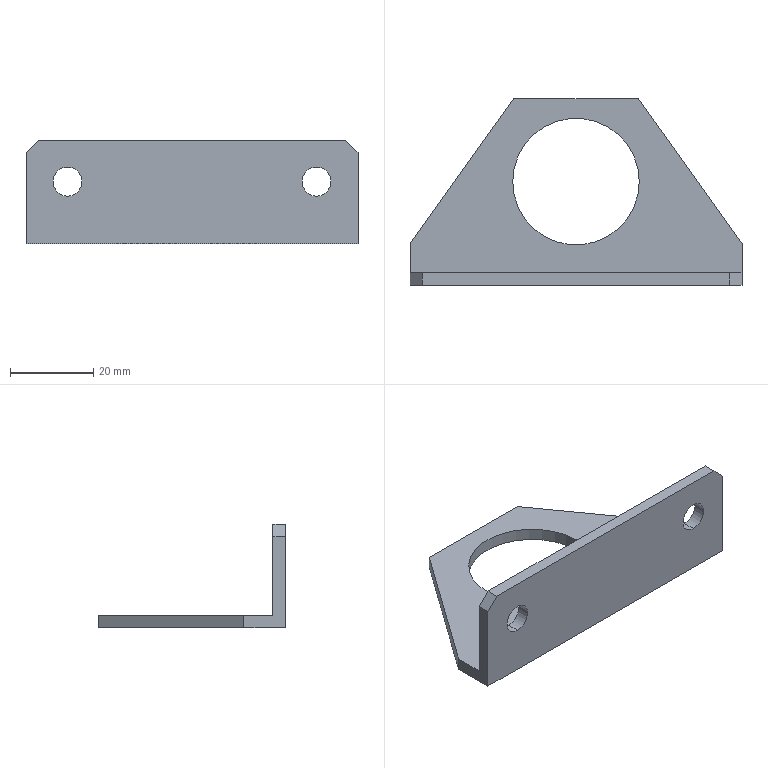Part | SolidWorks | features MBimport 1 | 1 solid | 18 faces | box 80 x 45 x 25 mm | volume 11005 mm3 | plane 12 | cylinder 6 | commonest cylinder face diameters 7 x4 30.5 x2
STEP:
#1=CARTESIAN_POINT('',(30.,3.,18.5));
#2=VERTEX_POINT('',#1);
#3=CARTESIAN_POINT('',(30.,0.,18.5));
#4=VERTEX_POINT('',#3);
#5=CARTESIAN_POINT('',(30.,3.,18.5));
#6=DIRECTION('',(0.,-1.,0.));
#7=VECTOR('',#6,1000.);
#8=LINE('',#5,#7);
#9=EDGE_CURVE('',#2,#4,#8,.T.);
#10=ORIENTED_EDGE('',*,*,#9,.F.);
#11=CARTESIAN_POINT('',(30.,3.,11.5));
#12=VERTEX_POINT('',#11);
#13=CARTESIAN_POINT('',(30.,3.,15.));
#14=DIRECTION('',(0.,-1.,0.));
#15=DIRECTION('',(0.,0.,-1.));
#16=AXIS2_PLACEMENT_3D('',#13,#14,#15);
#17=CIRCLE('',#16,3.5);
#18=EDGE_CURVE('',#12,#2,#17,.T.);
#19=ORIENTED_EDGE('',*,*,#18,.F.);
#20=CARTESIAN_POINT('',(30.,0.,11.5));
#21=VERTEX_POINT('',#20);
#22=CARTESIAN_POINT('',(30.,3.,11.5));
#23=DIRECTION('',(0.,-1.,0.));
#24=VECTOR('',#23,1000.);
#25=LINE('',#22,#24);
#26=EDGE_CURVE('',#12,#21,#25,.T.);
#27=ORIENTED_EDGE('',*,*,#26,.T.);
#28=CARTESIAN_POINT('',(30.,0.,15.));
#29=DIRECTION('',(0.,-1.,0.));
#30=DIRECTION('',(0.,0.,-1.));
#31=AXIS2_PLACEMENT_3D('',#28,#29,#30);
#32=CIRCLE('',#31,3.5);
#33=EDGE_CURVE('',#21,#4,#32,.T.);
#34=ORIENTED_EDGE('',*,*,#33,.T.);
#35=EDGE_LOOP('',(#10,#19,#27,#34));
#36=FACE_OUTER_BOUND('',#35,.T.);
#37=CARTESIAN_POINT('',(30.,3.,15.));
#38=DIRECTION('',(0.,-1.,0.));
#39=DIRECTION('',(0.,0.,-1.));
#40=AXIS2_PLACEMENT_3D('',#37,#38,#39);
#41=CYLINDRICAL_SURFACE('',#40,3.5);
#42=ADVANCED_FACE('',(#36),#41,.F.);
#43=CARTESIAN_POINT('',(-30.,3.,18.5));
#44=VERTEX_POINT('',#43);
#45=CARTESIAN_POINT('',(-30.,0.,18.5));
#46=VERTEX_POINT('',#45);
#47=CARTESIAN_POINT('',(-30.,3.,18.5));
#48=DIRECTION('',(0.,-1.,0.));
#49=VECTOR('',#48,1000.);
#50=LINE('',#47,#49);
#51=EDGE_CURVE('',#44,#46,#50,.T.);
#52=ORIENTED_EDGE('',*,*,#51,.F.);
#53=CARTESIAN_POINT('',(-30.,3.,11.5));
#54=VERTEX_POINT('',#53);
#55=CARTESIAN_POINT('',(-30.,3.,15.));
#56=DIRECTION('',(0.,-1.,0.));
#57=DIRECTION('',(0.,0.,-1.));
#58=AXIS2_PLACEMENT_3D('',#55,#56,#57);
#59=CIRCLE('',#58,3.5);
#60=EDGE_CURVE('',#54,#44,#59,.T.);
#61=ORIENTED_EDGE('',*,*,#60,.F.);
#62=CARTESIAN_POINT('',(-30.,0.,11.5));
#63=VERTEX_POINT('',#62);
#64=CARTESIAN_POINT('',(-30.,3.,11.5));
#65=DIRECTION('',(0.,-1.,0.));
#66=VECTOR('',#65,1000.);
#67=LINE('',#64,#66);
#68=EDGE_CURVE('',#54,#63,#67,.T.);
#69=ORIENTED_EDGE('',*,*,#68,.T.);
#70=CARTESIAN_POINT('',(-30.,0.,15.));
#71=DIRECTION('',(0.,-1.,0.));
#72=DIRECTION('',(0.,0.,-1.));
#73=AXIS2_PLACEMENT_3D('',#70,#71,#72);
#74=CIRCLE('',#73,3.5);
#75=EDGE_CURVE('',#63,#46,#74,.T.);
#76=ORIENTED_EDGE('',*,*,#75,.T.);
#77=EDGE_LOOP('',(#52,#61,#69,#76));
#78=FACE_OUTER_BOUND('',#77,.T.);
#79=CARTESIAN_POINT('',(-30.,3.,15.));
#80=DIRECTION('',(0.,-1.,0.));
#81=DIRECTION('',(0.,0.,-1.));
#82=AXIS2_PLACEMENT_3D('',#79,#80,#81);
#83=CYLINDRICAL_SURFACE('',#82,3.5);
#84=ADVANCED_FACE('',(#78),#83,.F.);
#85=ORIENTED_EDGE('',*,*,#60,.T.);
#86=CARTESIAN_POINT('',(-30.,3.,15.));
#87=DIRECTION('',(0.,-1.,0.));
#88=DIRECTION('',(0.,0.,-1.));
#89=AXIS2_PLACEMENT_3D('',#86,#87,#88);
#90=CIRCLE('',#89,3.5);
#91=EDGE_CURVE('',#44,#54,#90,.T.);
#92=ORIENTED_EDGE('',*,*,#91,.T.);
#93=EDGE_LOOP('',(#85,#92));
#94=FACE_BOUND('',#93,.T.);
#95=ORIENTED_EDGE('',*,*,#18,.T.);
#96=CARTESIAN_POINT('',(30.,3.,15.));
#97=DIRECTION('',(0.,-1.,0.));
#98=DIRECTION('',(0.,0.,-1.));
#99=AXIS2_PLACEMENT_3D('',#96,#97,#98);
#100=CIRCLE('',#99,3.5);
#101=EDGE_CURVE('',#2,#12,#100,.T.);
#102=ORIENTED_EDGE('',*,*,#101,.T.);
#103=EDGE_LOOP('',(#95,#102));
#104=FACE_BOUND('',#103,.T.);
#105=CARTESIAN_POINT('',(-40.,3.,3.));
#106=VERTEX_POINT('',#105);
#107=CARTESIAN_POINT('',(40.,3.,3.));
#108=VERTEX_POINT('',#107);
#109=CARTESIAN_POINT('',(0.,3.,3.));
#110=DIRECTION('',(1.,0.,0.));
#111=VECTOR('',#110,1000.);
#112=LINE('',#109,#111);
#113=EDGE_CURVE('',#106,#108,#112,.T.);
#114=ORIENTED_EDGE('',*,*,#113,.F.);
#115=CARTESIAN_POINT('',(-40.,3.,22.));
#116=VERTEX_POINT('',#115);
#117=CARTESIAN_POINT('',(-40.,3.,0.));
#118=DIRECTION('',(0.,0.,-1.));
#119=VECTOR('',#118,1000.);
#120=LINE('',#117,#119);
#121=EDGE_CURVE('',#116,#106,#120,.T.);
#122=ORIENTED_EDGE('',*,*,#121,.F.);
#123=CARTESIAN_POINT('',(-37.,3.,25.));
#124=VERTEX_POINT('',#123);
#125=CARTESIAN_POINT('',(-40.,3.,22.));
#126=DIRECTION('',(-0.7071,0.,-0.7071));
#127=VECTOR('',#126,1000.);
#128=LINE('',#125,#127);
#129=EDGE_CURVE('',#124,#116,#128,.T.);
#130=ORIENTED_EDGE('',*,*,#129,.F.);
#131=CARTESIAN_POINT('',(37.,3.,25.));
#132=VERTEX_POINT('',#131);
#133=CARTESIAN_POINT('',(-37.,3.,25.));
#134=DIRECTION('',(-1.,0.,0.));
#135=VECTOR('',#134,1000.);
#136=LINE('',#133,#135);
#137=EDGE_CURVE('',#132,#124,#136,.T.);
#138=ORIENTED_EDGE('',*,*,#137,.F.);
#139=CARTESIAN_POINT('',(40.,3.,22.));
#140=VERTEX_POINT('',#139);
#141=CARTESIAN_POINT('',(37.,3.,25.));
#142=DIRECTION('',(-0.7071,0.,0.7071));
#143=VECTOR('',#142,1000.);
#144=LINE('',#141,#143);
#145=EDGE_CURVE('',#140,#132,#144,.T.);
#146=ORIENTED_EDGE('',*,*,#145,.F.);
#147=CARTESIAN_POINT('',(40.,3.,0.));
#148=DIRECTION('',(0.,0.,1.));
#149=VECTOR('',#148,1000.);
#150=LINE('',#147,#149);
#151=EDGE_CURVE('',#108,#140,#150,.T.);
#152=ORIENTED_EDGE('',*,*,#151,.F.);
#153=EDGE_LOOP('',(#114,#122,#130,#138,#146,#152));
#154=FACE_OUTER_BOUND('',#153,.T.);
#155=CARTESIAN_POINT('',(0.,3.,0.));
#156=DIRECTION('',(0.,-1.,0.));
#157=DIRECTION('',(0.,0.,-1.));
#158=AXIS2_PLACEMENT_3D('',#155,#156,#157);
#159=PLANE('',#158);
#160=ADVANCED_FACE('',(#94,#104,#154),#159,.F.);
#161=CARTESIAN_POINT('',(40.,0.,22.));
#162=VERTEX_POINT('',#161);
#163=CARTESIAN_POINT('',(37.,0.,25.));
#164=VERTEX_POINT('',#163);
#165=CARTESIAN_POINT('',(37.,0.,25.));
#166=DIRECTION('',(-0.7071,0.,0.7071));
#167=VECTOR('',#166,1000.);
#168=LINE('',#165,#167);
#169=EDGE_CURVE('',#162,#164,#168,.T.);
#170=ORIENTED_EDGE('',*,*,#169,.F.);
#171=CARTESIAN_POINT('',(40.,3.,22.));
#172=DIRECTION('',(0.,-1.,0.));
#173=VECTOR('',#172,1000.);
#174=LINE('',#171,#173);
#175=EDGE_CURVE('',#140,#162,#174,.T.);
#176=ORIENTED_EDGE('',*,*,#175,.F.);
#177=ORIENTED_EDGE('',*,*,#145,.T.);
#178=CARTESIAN_POINT('',(37.,3.,25.));
#179=DIRECTION('',(0.,-1.,0.));
#180=VECTOR('',#179,1000.);
#181=LINE('',#178,#180);
#182=EDGE_CURVE('',#132,#164,#181,.T.);
#183=ORIENTED_EDGE('',*,*,#182,.T.);
#184=EDGE_LOOP('',(#170,#176,#177,#183));
#185=FACE_OUTER_BOUND('',#184,.T.);
#186=CARTESIAN_POINT('',(37.,3.,25.));
#187=DIRECTION('',(0.7071,0.,0.7071));
#188=DIRECTION('',(0.,-1.,0.));
#189=AXIS2_PLACEMENT_3D('',#186,#187,#188);
#190=PLANE('',#189);
#191=ADVANCED_FACE('',(#185),#190,.T.);
#192=CARTESIAN_POINT('',(-37.,0.,25.));
#193=VERTEX_POINT('',#192);
#194=CARTESIAN_POINT('',(-37.,0.,25.));
#195=DIRECTION('',(-1.,0.,0.));
#196=VECTOR('',#195,1000.);
#197=LINE('',#194,#196);
#198=EDGE_CURVE('',#164,#193,#197,.T.);
#199=ORIENTED_EDGE('',*,*,#198,.F.);
#200=ORIENTED_EDGE('',*,*,#182,.F.);
#201=ORIENTED_EDGE('',*,*,#137,.T.);
#202=CARTESIAN_POINT('',(-37.,3.,25.));
#203=DIRECTION('',(0.,-1.,0.));
#204=VECTOR('',#203,1000.);
#205=LINE('',#202,#204);
#206=EDGE_CURVE('',#124,#193,#205,.T.);
#207=ORIENTED_EDGE('',*,*,#206,.T.);
#208=EDGE_LOOP('',(#199,#200,#201,#207));
#209=FACE_OUTER_BOUND('',#208,.T.);
#210=CARTESIAN_POINT('',(-37.,3.,25.));
#211=DIRECTION('',(0.,0.,1.));
#212=DIRECTION('',(1.,0.,0.));
#213=AXIS2_PLACEMENT_3D('',#210,#211,#212);
#214=PLANE('',#213);
#215=ADVANCED_FACE('',(#209),#214,.T.);
#216=CARTESIAN_POINT('',(-40.,0.,22.));
#217=VERTEX_POINT('',#216);
#218=CARTESIAN_POINT('',(-40.,0.,22.));
#219=DIRECTION('',(-0.7071,0.,-0.7071));
#220=VECTOR('',#219,1000.);
#221=LINE('',#218,#220);
#222=EDGE_CURVE('',#193,#217,#221,.T.);
#223=ORIENTED_EDGE('',*,*,#222,.F.);
#224=ORIENTED_EDGE('',*,*,#206,.F.);
#225=ORIENTED_EDGE('',*,*,#129,.T.);
#226=CARTESIAN_POINT('',(-40.,3.,22.));
#227=DIRECTION('',(0.,-1.,0.));
#228=VECTOR('',#227,1000.);
#229=LINE('',#226,#228);
#230=EDGE_CURVE('',#116,#217,#229,.T.);
#231=ORIENTED_EDGE('',*,*,#230,.T.);
#232=EDGE_LOOP('',(#223,#224,#225,#231));
#233=FACE_OUTER_BOUND('',#232,.T.);
#234=CARTESIAN_POINT('',(-40.,3.,22.));
#235=DIRECTION('',(-0.7071,0.,0.7071));
#236=DIRECTION('',(0.,1.,0.));
#237=AXIS2_PLACEMENT_3D('',#234,#235,#236);
#238=PLANE('',#237);
#239=ADVANCED_FACE('',(#233),#238,.T.);
#240=CARTESIAN_POINT('',(15.25,25.,3.));
#241=VERTEX_POINT('',#240);
#242=CARTESIAN_POINT('',(15.25,25.,0.));
#243=VERTEX_POINT('',#242);
#244=CARTESIAN_POINT('',(15.25,25.,3.));
#245=DIRECTION('',(0.,0.,-1.));
#246=VECTOR('',#245,1000.);
#247=LINE('',#244,#246);
#248=EDGE_CURVE('',#241,#243,#247,.T.);
#249=ORIENTED_EDGE('',*,*,#248,.F.);
#250=CARTESIAN_POINT('',(-15.25,25.,3.));
#251=VERTEX_POINT('',#250);
#252=CARTESIAN_POINT('',(0.,25.,3.));
#253=DIRECTION('',(0.,0.,1.));
#254=DIRECTION('',(1.,0.,0.));
#255=AXIS2_PLACEMENT_3D('',#252,#253,#254);
#256=CIRCLE('',#255,15.25);
#257=EDGE_CURVE('',#241,#251,#256,.T.);
#258=ORIENTED_EDGE('',*,*,#257,.T.);
#259=CARTESIAN_POINT('',(-15.25,25.,0.));
#260=VERTEX_POINT('',#259);
#261=CARTESIAN_POINT('',(-15.25,25.,3.));
#262=DIRECTION('',(0.,0.,-1.));
#263=VECTOR('',#262,1000.);
#264=LINE('',#261,#263);
#265=EDGE_CURVE('',#251,#260,#264,.T.);
#266=ORIENTED_EDGE('',*,*,#265,.T.);
#267=CARTESIAN_POINT('',(0.,25.,0.));
#268=DIRECTION('',(0.,0.,1.));
#269=DIRECTION('',(1.,0.,0.));
#270=AXIS2_PLACEMENT_3D('',#267,#268,#269);
#271=CIRCLE('',#270,15.25);
#272=EDGE_CURVE('',#243,#260,#271,.T.);
#273=ORIENTED_EDGE('',*,*,#272,.F.);
#274=EDGE_LOOP('',(#249,#258,#266,#273));
#275=FACE_OUTER_BOUND('',#274,.T.);
#276=CARTESIAN_POINT('',(0.,25.,3.));
#277=DIRECTION('',(0.,0.,-1.));
#278=DIRECTION('',(-1.,0.,0.));
#279=AXIS2_PLACEMENT_3D('',#276,#277,#278);
#280=CYLINDRICAL_SURFACE('',#279,15.25);
#281=ADVANCED_FACE('',(#275),#280,.F.);
#282=CARTESIAN_POINT('',(-15.,45.,0.));
#283=VERTEX_POINT('',#282);
#284=CARTESIAN_POINT('',(-40.,10.,0.));
#285=VERTEX_POINT('',#284);
#286=CARTESIAN_POINT('',(-15.,45.,0.));
#287=DIRECTION('',(-0.5812,-0.8137,0.));
#288=VECTOR('',#287,1000.);
#289=LINE('',#286,#288);
#290=EDGE_CURVE('',#283,#285,#289,.T.);
#291=ORIENTED_EDGE('',*,*,#290,.T.);
#292=CARTESIAN_POINT('',(-40.,10.,3.));
#293=VERTEX_POINT('',#292);
#294=CARTESIAN_POINT('',(-40.,10.,3.));
#295=DIRECTION('',(0.,0.,-1.));
#296=VECTOR('',#295,1000.);
#297=LINE('',#294,#296);
#298=EDGE_CURVE('',#293,#285,#297,.T.);
#299=ORIENTED_EDGE('',*,*,#298,.F.);
#300=CARTESIAN_POINT('',(-15.,45.,3.));
#301=VERTEX_POINT('',#300);
#302=CARTESIAN_POINT('',(-15.,45.,3.));
#303=DIRECTION('',(-0.5812,-0.8137,0.));
#304=VECTOR('',#303,1000.);
#305=LINE('',#302,#304);
#306=EDGE_CURVE('',#301,#293,#305,.T.);
#307=ORIENTED_EDGE('',*,*,#306,.F.);
#308=CARTESIAN_POINT('',(-15.,45.,3.));
#309=DIRECTION('',(0.,0.,-1.));
#310=VECTOR('',#309,1000.);
#311=LINE('',#308,#310);
#312=EDGE_CURVE('',#301,#283,#311,.T.);
#313=ORIENTED_EDGE('',*,*,#312,.T.);
#314=EDGE_LOOP('',(#291,#299,#307,#313));
#315=FACE_OUTER_BOUND('',#314,.T.);
#316=CARTESIAN_POINT('',(-15.,45.,3.));
#317=DIRECTION('',(0.8137,-0.5812,0.));
#318=DIRECTION('',(0.,0.,-1.));
#319=AXIS2_PLACEMENT_3D('',#316,#317,#318);
#320=PLANE('',#319);
#321=ADVANCED_FACE('',(#315),#320,.F.);
#322=CARTESIAN_POINT('',(15.,45.,0.));
#323=VERTEX_POINT('',#322);
#324=CARTESIAN_POINT('',(15.,45.,0.));
#325=DIRECTION('',(-1.,0.,0.));
#326=VECTOR('',#325,1000.);
#327=LINE('',#324,#326);
#328=EDGE_CURVE('',#323,#283,#327,.T.);
#329=ORIENTED_EDGE('',*,*,#328,.T.);
#330=ORIENTED_EDGE('',*,*,#312,.F.);
#331=CARTESIAN_POINT('',(15.,45.,3.));
#332=VERTEX_POINT('',#331);
#333=CARTESIAN_POINT('',(15.,45.,3.));
#334=DIRECTION('',(-1.,0.,0.));
#335=VECTOR('',#334,1000.);
#336=LINE('',#333,#335);
#337=EDGE_CURVE('',#332,#301,#336,.T.);
#338=ORIENTED_EDGE('',*,*,#337,.F.);
#339=CARTESIAN_POINT('',(15.,45.,3.));
#340=DIRECTION('',(0.,0.,-1.));
#341=VECTOR('',#340,1000.);
#342=LINE('',#339,#341);
#343=EDGE_CURVE('',#332,#323,#342,.T.);
#344=ORIENTED_EDGE('',*,*,#343,.T.);
#345=EDGE_LOOP('',(#329,#330,#338,#344));
#346=FACE_OUTER_BOUND('',#345,.T.);
#347=CARTESIAN_POINT('',(15.,45.,3.));
#348=DIRECTION('',(0.,-1.,0.));
#349=DIRECTION('',(0.,0.,-1.));
#350=AXIS2_PLACEMENT_3D('',#347,#348,#349);
#351=PLANE('',#350);
#352=ADVANCED_FACE('',(#346),#351,.F.);
#353=CARTESIAN_POINT('',(40.,10.,0.));
#354=VERTEX_POINT('',#353);
#355=CARTESIAN_POINT('',(40.,10.,0.));
#356=DIRECTION('',(-0.5812,0.8137,0.));
#357=VECTOR('',#356,1000.);
#358=LINE('',#355,#357);
#359=EDGE_CURVE('',#354,#323,#358,.T.);
#360=ORIENTED_EDGE('',*,*,#359,.T.);
#361=ORIENTED_EDGE('',*,*,#343,.F.);
#362=CARTESIAN_POINT('',(40.,10.,3.));
#363=VERTEX_POINT('',#362);
#364=CARTESIAN_POINT('',(40.,10.,3.));
#365=DIRECTION('',(-0.5812,0.8137,0.));
#366=VECTOR('',#365,1000.);
#367=LINE('',#364,#366);
#368=EDGE_CURVE('',#363,#332,#367,.T.);
#369=ORIENTED_EDGE('',*,*,#368,.F.);
#370=CARTESIAN_POINT('',(40.,10.,3.));
#371=DIRECTION('',(0.,0.,-1.));
#372=VECTOR('',#371,1000.);
#373=LINE('',#370,#372);
#374=EDGE_CURVE('',#363,#354,#373,.T.);
#375=ORIENTED_EDGE('',*,*,#374,.T.);
#376=EDGE_LOOP('',(#360,#361,#369,#375));
#377=FACE_OUTER_BOUND('',#376,.T.);
#378=CARTESIAN_POINT('',(40.,10.,3.));
#379=DIRECTION('',(-0.8137,-0.5812,0.));
#380=DIRECTION('',(-0.5812,0.8137,0.));
#381=AXIS2_PLACEMENT_3D('',#378,#379,#380);
#382=PLANE('',#381);
#383=ADVANCED_FACE('',(#377),#382,.F.);
#384=CARTESIAN_POINT('',(40.,0.,0.));
#385=VERTEX_POINT('',#384);
#386=CARTESIAN_POINT('',(40.,0.,0.));
#387=DIRECTION('',(0.,1.,0.));
#388=VECTOR('',#387,1000.);
#389=LINE('',#386,#388);
#390=EDGE_CURVE('',#385,#354,#389,.T.);
#391=ORIENTED_EDGE('',*,*,#390,.T.);
#392=ORIENTED_EDGE('',*,*,#374,.F.);
#393=CARTESIAN_POINT('',(40.,0.,3.));
#394=DIRECTION('',(0.,1.,0.));
#395=VECTOR('',#394,1000.);
#396=LINE('',#393,#395);
#397=EDGE_CURVE('',#108,#363,#396,.T.);
#398=ORIENTED_EDGE('',*,*,#397,.F.);
#399=ORIENTED_EDGE('',*,*,#151,.T.);
#400=ORIENTED_EDGE('',*,*,#175,.T.);
#401=CARTESIAN_POINT('',(40.,0.,3.));
#402=DIRECTION('',(0.,0.,-1.));
#403=VECTOR('',#402,1000.);
#404=LINE('',#401,#403);
#405=EDGE_CURVE('',#162,#385,#404,.T.);
#406=ORIENTED_EDGE('',*,*,#405,.T.);
#407=EDGE_LOOP('',(#391,#392,#398,#399,#400,#406));
#408=FACE_OUTER_BOUND('',#407,.T.);
#409=CARTESIAN_POINT('',(40.,0.,3.));
#410=DIRECTION('',(-1.,0.,0.));
#411=DIRECTION('',(0.,0.,1.));
#412=AXIS2_PLACEMENT_3D('',#409,#410,#411);
#413=PLANE('',#412);
#414=ADVANCED_FACE('',(#408),#413,.F.);
#415=ORIENTED_EDGE('',*,*,#75,.F.);
#416=CARTESIAN_POINT('',(-30.,0.,15.));
#417=DIRECTION('',(0.,-1.,0.));
#418=DIRECTION('',(0.,0.,-1.));
#419=AXIS2_PLACEMENT_3D('',#416,#417,#418);
#420=CIRCLE('',#419,3.5);
#421=EDGE_CURVE('',#46,#63,#420,.T.);
#422=ORIENTED_EDGE('',*,*,#421,.F.);
#423=EDGE_LOOP('',(#415,#422));
#424=FACE_BOUND('',#423,.T.);
#425=ORIENTED_EDGE('',*,*,#33,.F.);
#426=CARTESIAN_POINT('',(30.,0.,15.));
#427=DIRECTION('',(0.,-1.,0.));
#428=DIRECTION('',(0.,0.,-1.));
#429=AXIS2_PLACEMENT_3D('',#426,#427,#428);
#430=CIRCLE('',#429,3.5);
#431=EDGE_CURVE('',#4,#21,#430,.T.);
#432=ORIENTED_EDGE('',*,*,#431,.F.);
#433=EDGE_LOOP('',(#425,#432));
#434=FACE_BOUND('',#433,.T.);
#435=CARTESIAN_POINT('',(-40.,0.,0.));
#436=VERTEX_POINT('',#435);
#437=CARTESIAN_POINT('',(-40.,0.,0.));
#438=DIRECTION('',(1.,0.,0.));
#439=VECTOR('',#438,1000.);
#440=LINE('',#437,#439);
#441=EDGE_CURVE('',#436,#385,#440,.T.);
#442=ORIENTED_EDGE('',*,*,#441,.T.);
#443=ORIENTED_EDGE('',*,*,#405,.F.);
#444=ORIENTED_EDGE('',*,*,#169,.T.);
#445=ORIENTED_EDGE('',*,*,#198,.T.);
#446=ORIENTED_EDGE('',*,*,#222,.T.);
#447=CARTESIAN_POINT('',(-40.,0.,3.));
#448=DIRECTION('',(0.,0.,-1.));
#449=VECTOR('',#448,1000.);
#450=LINE('',#447,#449);
#451=EDGE_CURVE('',#217,#436,#450,.T.);
#452=ORIENTED_EDGE('',*,*,#451,.T.);
#453=EDGE_LOOP('',(#442,#443,#444,#445,#446,#452));
#454=FACE_OUTER_BOUND('',#453,.T.);
#455=CARTESIAN_POINT('',(-40.,0.,3.));
#456=DIRECTION('',(0.,1.,0.));
#457=DIRECTION('',(1.,0.,0.));
#458=AXIS2_PLACEMENT_3D('',#455,#456,#457);
#459=PLANE('',#458);
#460=ADVANCED_FACE('',(#424,#434,#454),#459,.F.);
#461=ORIENTED_EDGE('',*,*,#451,.F.);
#462=ORIENTED_EDGE('',*,*,#230,.F.);
#463=ORIENTED_EDGE('',*,*,#121,.T.);
#464=CARTESIAN_POINT('',(-40.,10.,3.));
#465=DIRECTION('',(0.,-1.,0.));
#466=VECTOR('',#465,1000.);
#467=LINE('',#464,#466);
#468=EDGE_CURVE('',#293,#106,#467,.T.);
#469=ORIENTED_EDGE('',*,*,#468,.F.);
#470=ORIENTED_EDGE('',*,*,#298,.T.);
#471=CARTESIAN_POINT('',(-40.,10.,0.));
#472=DIRECTION('',(0.,-1.,0.));
#473=VECTOR('',#472,1000.);
#474=LINE('',#471,#473);
#475=EDGE_CURVE('',#285,#436,#474,.T.);
#476=ORIENTED_EDGE('',*,*,#475,.T.);
#477=EDGE_LOOP('',(#461,#462,#463,#469,#470,#476));
#478=FACE_OUTER_BOUND('',#477,.T.);
#479=CARTESIAN_POINT('',(-40.,10.,3.));
#480=DIRECTION('',(1.,0.,0.));
#481=DIRECTION('',(0.,1.,0.));
#482=AXIS2_PLACEMENT_3D('',#479,#480,#481);
#483=PLANE('',#482);
#484=ADVANCED_FACE('',(#478),#483,.F.);
#485=CARTESIAN_POINT('',(0.,25.,0.));
#486=DIRECTION('',(0.,0.,1.));
#487=DIRECTION('',(1.,0.,0.));
#488=AXIS2_PLACEMENT_3D('',#485,#486,#487);
#489=CIRCLE('',#488,15.25);
#490=EDGE_CURVE('',#260,#243,#489,.T.);
#491=ORIENTED_EDGE('',*,*,#490,.T.);
#492=ORIENTED_EDGE('',*,*,#272,.T.);
#493=EDGE_LOOP('',(#491,#492));
#494=FACE_BOUND('',#493,.T.);
#495=ORIENTED_EDGE('',*,*,#441,.F.);
#496=ORIENTED_EDGE('',*,*,#475,.F.);
#497=ORIENTED_EDGE('',*,*,#290,.F.);
#498=ORIENTED_EDGE('',*,*,#328,.F.);
#499=ORIENTED_EDGE('',*,*,#359,.F.);
#500=ORIENTED_EDGE('',*,*,#390,.F.);
#501=EDGE_LOOP('',(#495,#496,#497,#498,#499,#500));
#502=FACE_OUTER_BOUND('',#501,.T.);
#503=CARTESIAN_POINT('',(0.,0.,0.));
#504=DIRECTION('',(0.,0.,1.));
#505=DIRECTION('',(1.,0.,0.));
#506=AXIS2_PLACEMENT_3D('',#503,#504,#505);
#507=PLANE('',#506);
#508=ADVANCED_FACE('',(#494,#502),#507,.F.);
#509=CARTESIAN_POINT('',(0.,25.,3.));
#510=DIRECTION('',(0.,0.,1.));
#511=DIRECTION('',(1.,0.,0.));
#512=AXIS2_PLACEMENT_3D('',#509,#510,#511);
#513=CIRCLE('',#512,15.25);
#514=EDGE_CURVE('',#251,#241,#513,.T.);
#515=ORIENTED_EDGE('',*,*,#514,.F.);
#516=ORIENTED_EDGE('',*,*,#257,.F.);
#517=EDGE_LOOP('',(#515,#516));
#518=FACE_BOUND('',#517,.T.);
#519=ORIENTED_EDGE('',*,*,#468,.T.);
#520=ORIENTED_EDGE('',*,*,#113,.T.);
#521=ORIENTED_EDGE('',*,*,#397,.T.);
#522=ORIENTED_EDGE('',*,*,#368,.T.);
#523=ORIENTED_EDGE('',*,*,#337,.T.);
#524=ORIENTED_EDGE('',*,*,#306,.T.);
#525=EDGE_LOOP('',(#519,#520,#521,#522,#523,#524));
#526=FACE_OUTER_BOUND('',#525,.T.);
#527=CARTESIAN_POINT('',(0.,0.,3.));
#528=DIRECTION('',(0.,0.,1.));
#529=DIRECTION('',(1.,0.,0.));
#530=AXIS2_PLACEMENT_3D('',#527,#528,#529);
#531=PLANE('',#530);
#532=ADVANCED_FACE('',(#518,#526),#531,.T.);
#533=ORIENTED_EDGE('',*,*,#514,.T.);
#534=ORIENTED_EDGE('',*,*,#248,.T.);
#535=ORIENTED_EDGE('',*,*,#490,.F.);
#536=ORIENTED_EDGE('',*,*,#265,.F.);
#537=EDGE_LOOP('',(#533,#534,#535,#536));
#538=FACE_OUTER_BOUND('',#537,.T.);
#539=CARTESIAN_POINT('',(0.,25.,3.));
#540=DIRECTION('',(0.,0.,-1.));
#541=DIRECTION('',(-1.,0.,0.));
#542=AXIS2_PLACEMENT_3D('',#539,#540,#541);
#543=CYLINDRICAL_SURFACE('',#542,15.25);
#544=ADVANCED_FACE('',(#538),#543,.F.);
#545=ORIENTED_EDGE('',*,*,#91,.F.);
#546=ORIENTED_EDGE('',*,*,#51,.T.);
#547=ORIENTED_EDGE('',*,*,#421,.T.);
#548=ORIENTED_EDGE('',*,*,#68,.F.);
#549=EDGE_LOOP('',(#545,#546,#547,#548));
#550=FACE_OUTER_BOUND('',#549,.T.);
#551=CARTESIAN_POINT('',(-30.,3.,15.));
#552=DIRECTION('',(0.,-1.,0.));
#553=DIRECTION('',(0.,0.,-1.));
#554=AXIS2_PLACEMENT_3D('',#551,#552,#553);
#555=CYLINDRICAL_SURFACE('',#554,3.5);
#556=ADVANCED_FACE('',(#550),#555,.F.);
#557=ORIENTED_EDGE('',*,*,#101,.F.);
#558=ORIENTED_EDGE('',*,*,#9,.T.);
#559=ORIENTED_EDGE('',*,*,#431,.T.);
#560=ORIENTED_EDGE('',*,*,#26,.F.);
#561=EDGE_LOOP('',(#557,#558,#559,#560));
#562=FACE_OUTER_BOUND('',#561,.T.);
#563=CARTESIAN_POINT('',(30.,3.,15.));
#564=DIRECTION('',(0.,-1.,0.));
#565=DIRECTION('',(0.,0.,-1.));
#566=AXIS2_PLACEMENT_3D('',#563,#564,#565);
#567=CYLINDRICAL_SURFACE('',#566,3.5);
#568=ADVANCED_FACE('',(#562),#567,.F.);
#569=CLOSED_SHELL('',(#42,#84,#160,#191,#215,#239,#281,#321,#352,#383,#414,#460,#484,#508,#532,#544,#556,#568));
#570=MANIFOLD_SOLID_BREP('',#569);
#571=CARTESIAN_POINT('',(0.,0.,0.));
#572=DIRECTION('',(0.,0.,1.));
#573=DIRECTION('',(1.,0.,0.));
#574=AXIS2_PLACEMENT_3D('',#571,#572,#573);
#575=(LENGTH_UNIT()NAMED_UNIT(*)SI_UNIT(.MILLI.,.METRE.));
#576=UNCERTAINTY_MEASURE_WITH_UNIT(LENGTH_MEASURE(0.00001),#575,'','');
#577=(NAMED_UNIT(*)PLANE_ANGLE_UNIT()SI_UNIT($,.RADIAN.));
#578=(NAMED_UNIT(*)SI_UNIT($,.STERADIAN.)SOLID_ANGLE_UNIT());
#579=(GEOMETRIC_REPRESENTATION_CONTEXT(3)GLOBAL_UNCERTAINTY_ASSIGNED_CONTEXT((#576))GLOBAL_UNIT_ASSIGNED_CONTEXT((#575,#577,#578))REPRESENTATION_CONTEXT('',''));
#580=ADVANCED_BREP_SHAPE_REPRESENTATION('',(#570,#574),#579);